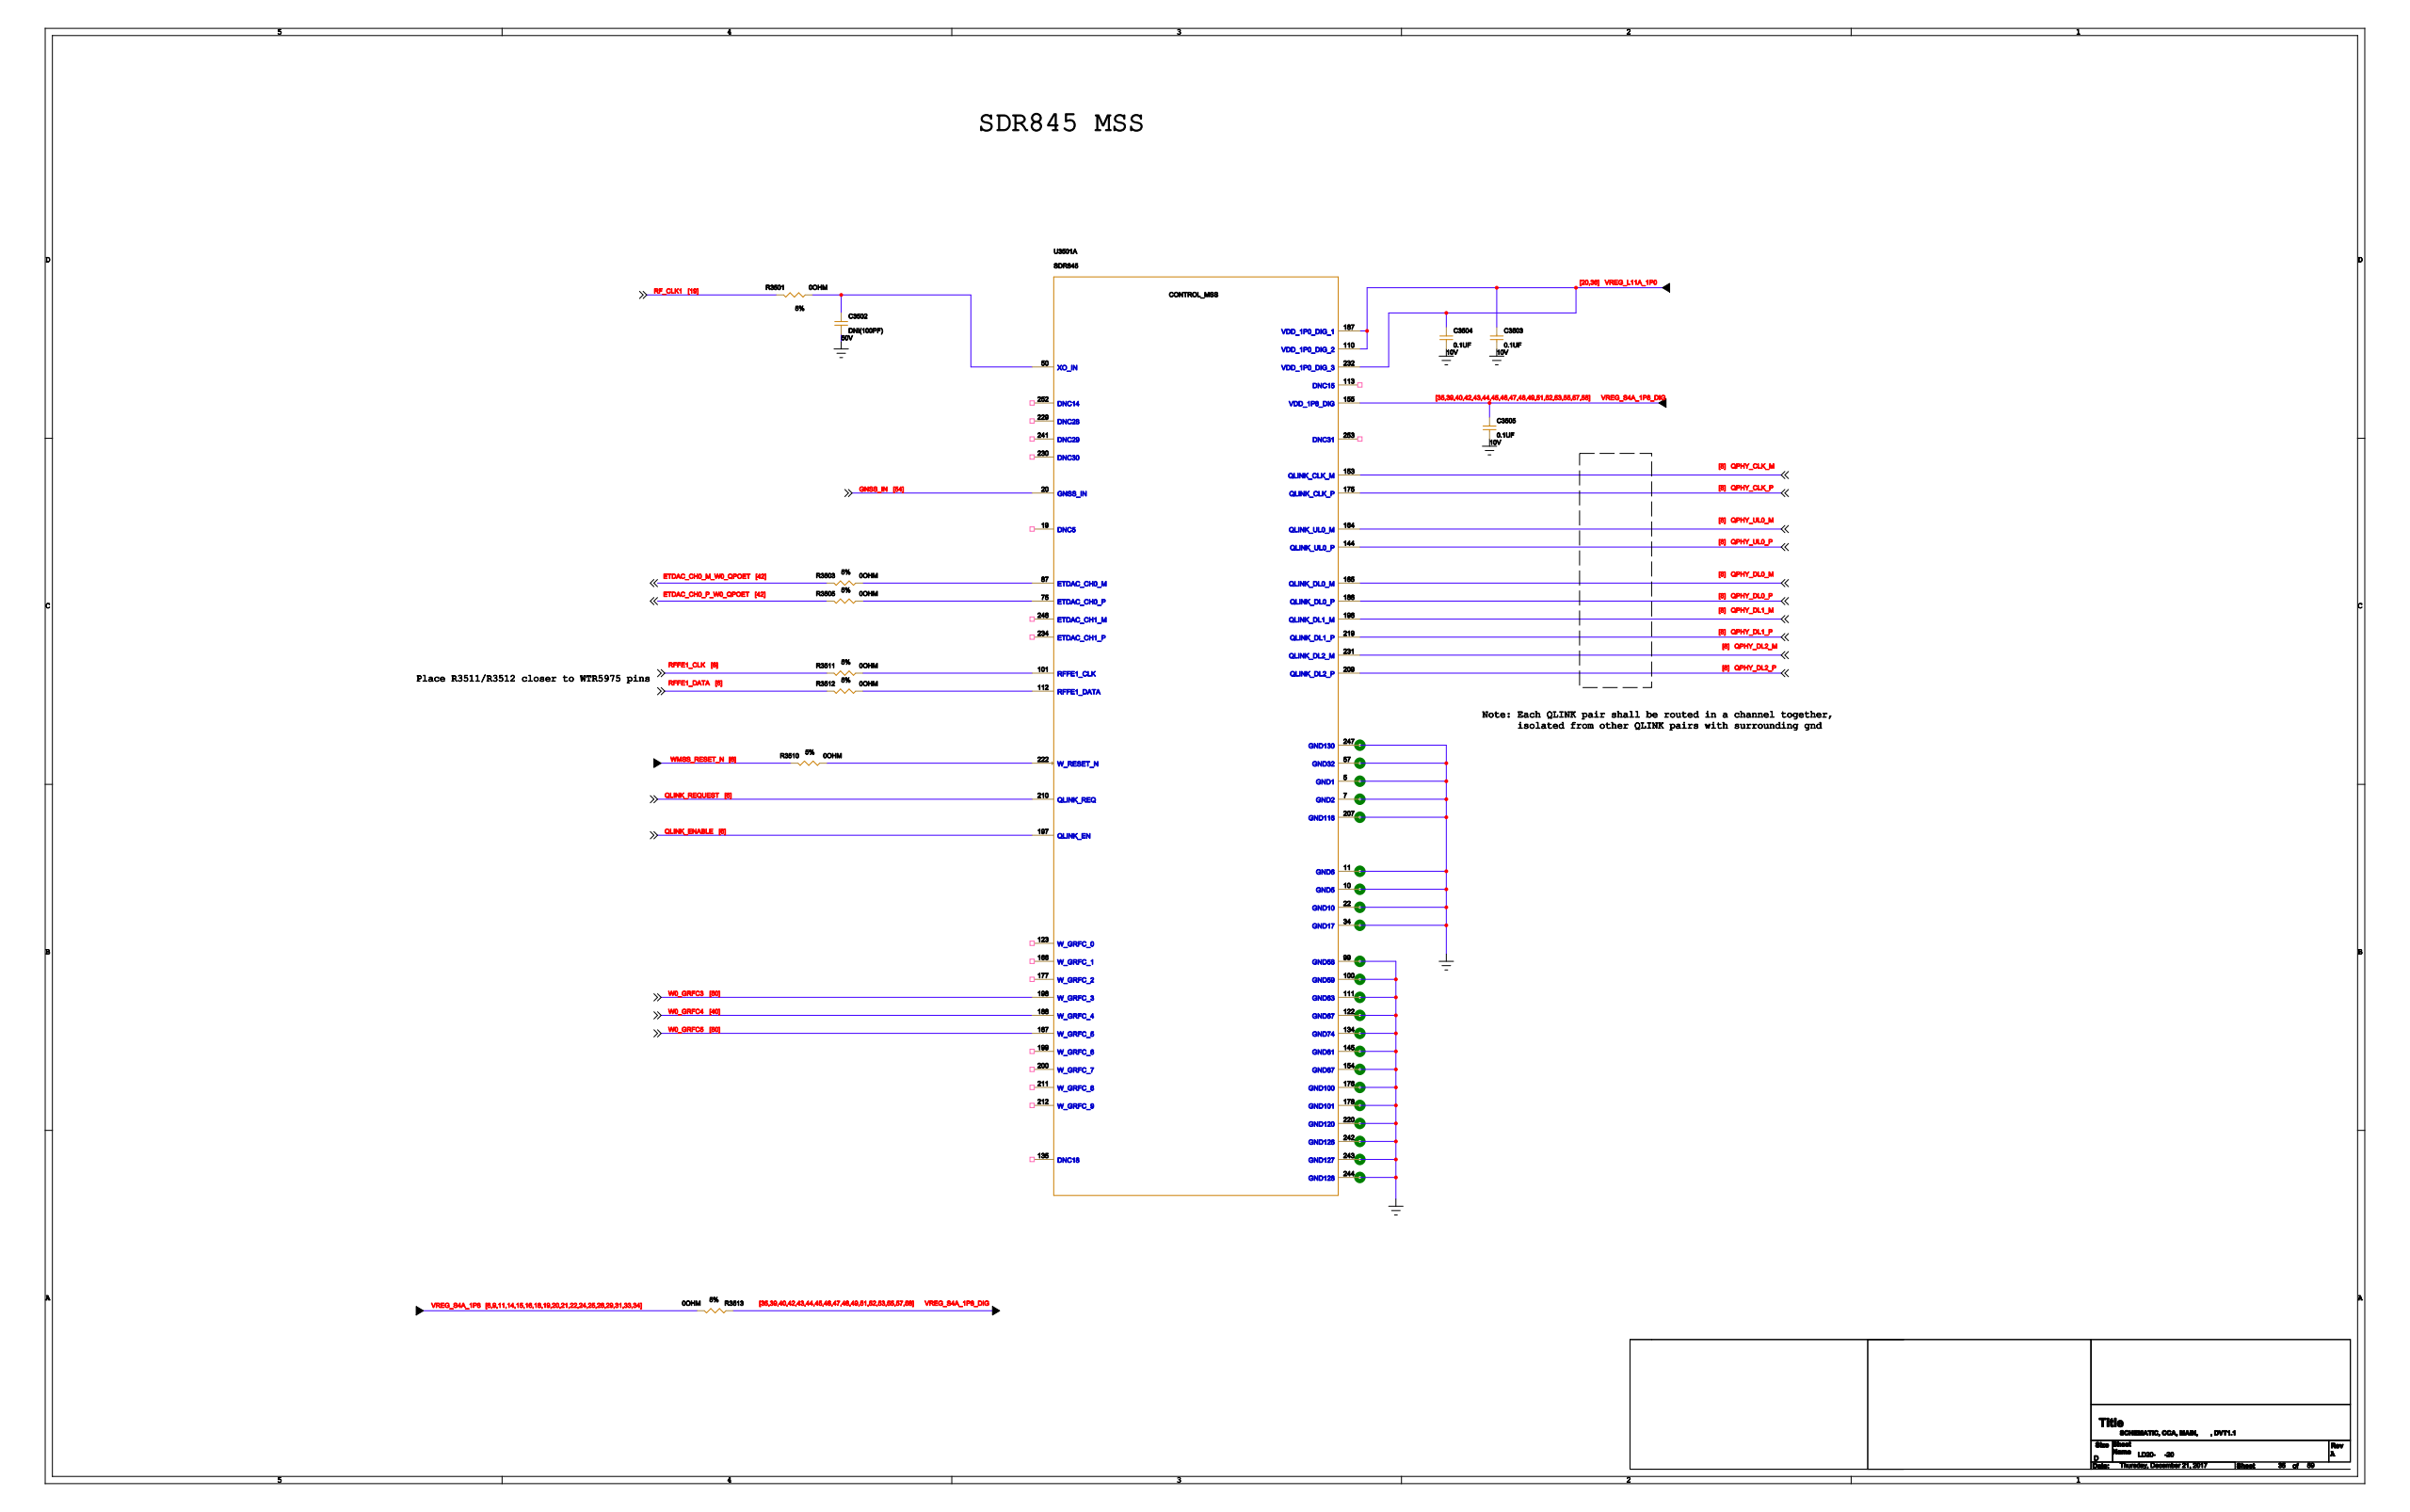Circuit board | Cadence Allegro | 1520 parts | 1149 nets | one sheet of the schematic
Parts on this sheet (reference | value | footprint):
C3502 | DNI(100PF) | 2P0201R_DNI
C3503 | 0.1UF | 2P0201R
C3504 | 0.1UF | 2P0201R
C3505 | 0.1UF | 2P0201R
R3501 | 0OHM | 2P0201R
R3503 | 0OHM | 2P0201R
R3505 | 0OHM | 2P0201R
R3510 | 0OHM | 2P0201R
R3511 | 0OHM | 2P0201R
R3512 | 0OHM | 2P0201R
R3513 | 0OHM | 2P0201R
U3501 | SDR845 | 253PGA235X247B138D45
Nets of these parts (net: part-pin ...):
GND: C3502-2 C3503-2 C3504-2 C3505-2 U3501-5 U3501-7 U3501-9 U3501-10 U3501-11 U3501-14 U3501-21 U3501-22 U3501-25 U3501-26 U3501-29 U3501-33 U3501-34 U3501-39 U3501-40 U3501-42 U3501-43 U3501-45 U3501-46 U3501-47 U3501-48 U3501-52 U3501-53 U3501-55 U3501-57 U3501-59 U3501-99 U3501-100 U3501-111 U3501-122 U3501-134 U3501-145 U3501-154 U3501-176 U3501-178 U3501-207 U3501-220 U3501-242 U3501-243 U3501-244 U3501-247
VREG_S4A_1P8: R3513-2
VREG_S4A_1P8_DIG: C3505-1 R3513-1 U3501-155
N33723779: R3503-2 U3501-87
N33724097: R3505-2 U3501-75
GNSS_IN: U3501-20
QPHY_CLK_M: U3501-153
QPHY_CLK_P: U3501-175
QPHY_DL0_M: U3501-165
QPHY_DL0_P: U3501-186
QPHY_DL1_M: U3501-196
QPHY_DL1_P: U3501-219
QPHY_DL2_M: U3501-231
QPHY_DL2_P: U3501-209
QLINK_ENABLE: U3501-197
QLINK_REQUEST: U3501-210
QPHY_UL0_M: U3501-164
QPHY_UL0_P: U3501-144
N35667619: R3511-2 U3501-101
N35664942: R3512-2 U3501-112
VREG_L11A_1P0: C3503-1 C3504-1 U3501-110 U3501-187 U3501-232
W0_GRFC3: U3501-198
W0_GRFC4: U3501-188
W0_GRFC5: U3501-167
N34547171: R3510-2 U3501-222
N30833962: C3502-1 R3501-2 U3501-50
RF_CLK1: R3501-1
ETDAC_CH0_M_W0_QPOET: R3503-1
ETDAC_CH0_P_W0_QPOET: R3505-1
WMSS_RESET_N: R3510-1
RFFE1_CLK: R3511-1
RFFE1_DATA: R3512-1